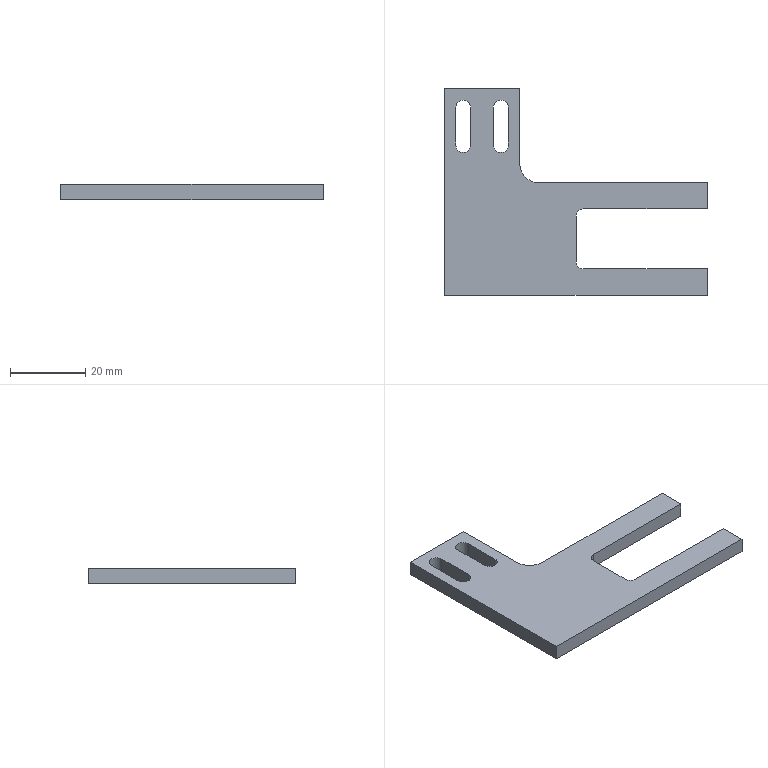Part | SolidWorks | features Fillet 2, ICE 2, Extrusion 1 | 1 solid | 23 faces | box 70 x 55 x 4 mm | volume 7768 mm3 | plane 16 | cylinder 7 | commonest cylinder face diameters 4 x6 10 x1
STEP:
#1=CARTESIAN_POINT('',(70.,-55.,0.));
#2=VERTEX_POINT('',#1);
#3=CARTESIAN_POINT('',(70.,-48.,0.));
#4=VERTEX_POINT('',#3);
#5=CARTESIAN_POINT('',(70.,-55.,0.));
#6=DIRECTION('',(0.,1.,0.));
#7=VECTOR('',#6,1000.);
#8=LINE('',#5,#7);
#9=EDGE_CURVE('',#2,#4,#8,.T.);
#10=ORIENTED_EDGE('',*,*,#9,.T.);
#11=CARTESIAN_POINT('',(70.,-48.,4.));
#12=VERTEX_POINT('',#11);
#13=CARTESIAN_POINT('',(70.,-48.,-0.001));
#14=DIRECTION('',(0.,0.,1.));
#15=VECTOR('',#14,1000.);
#16=LINE('',#13,#15);
#17=EDGE_CURVE('',#4,#12,#16,.T.);
#18=ORIENTED_EDGE('',*,*,#17,.T.);
#19=CARTESIAN_POINT('',(70.,-55.,4.));
#20=VERTEX_POINT('',#19);
#21=CARTESIAN_POINT('',(70.,-55.,4.));
#22=DIRECTION('',(0.,1.,0.));
#23=VECTOR('',#22,1000.);
#24=LINE('',#21,#23);
#25=EDGE_CURVE('',#20,#12,#24,.T.);
#26=ORIENTED_EDGE('',*,*,#25,.F.);
#27=CARTESIAN_POINT('',(70.,-55.,4.));
#28=DIRECTION('',(0.,0.,-1.));
#29=VECTOR('',#28,1000.);
#30=LINE('',#27,#29);
#31=EDGE_CURVE('',#20,#2,#30,.T.);
#32=ORIENTED_EDGE('',*,*,#31,.T.);
#33=EDGE_LOOP('',(#10,#18,#26,#32));
#34=FACE_OUTER_BOUND('',#33,.T.);
#35=CARTESIAN_POINT('',(70.,-55.,4.));
#36=DIRECTION('',(-1.,0.,0.));
#37=DIRECTION('',(0.,0.,1.));
#38=AXIS2_PLACEMENT_3D('',#35,#36,#37);
#39=PLANE('',#38);
#40=ADVANCED_FACE('',(#34),#39,.F.);
#41=CARTESIAN_POINT('',(20.,0.,0.));
#42=VERTEX_POINT('',#41);
#43=CARTESIAN_POINT('',(0.,0.,0.));
#44=VERTEX_POINT('',#43);
#45=CARTESIAN_POINT('',(20.,0.,0.));
#46=DIRECTION('',(-1.,0.,0.));
#47=VECTOR('',#46,1000.);
#48=LINE('',#45,#47);
#49=EDGE_CURVE('',#42,#44,#48,.T.);
#50=ORIENTED_EDGE('',*,*,#49,.T.);
#51=CARTESIAN_POINT('',(0.,0.,4.));
#52=VERTEX_POINT('',#51);
#53=CARTESIAN_POINT('',(0.,0.,4.));
#54=DIRECTION('',(0.,0.,-1.));
#55=VECTOR('',#54,1000.);
#56=LINE('',#53,#55);
#57=EDGE_CURVE('',#52,#44,#56,.T.);
#58=ORIENTED_EDGE('',*,*,#57,.F.);
#59=CARTESIAN_POINT('',(20.,0.,4.));
#60=VERTEX_POINT('',#59);
#61=CARTESIAN_POINT('',(20.,0.,4.));
#62=DIRECTION('',(-1.,0.,0.));
#63=VECTOR('',#62,1000.);
#64=LINE('',#61,#63);
#65=EDGE_CURVE('',#60,#52,#64,.T.);
#66=ORIENTED_EDGE('',*,*,#65,.F.);
#67=CARTESIAN_POINT('',(20.,0.,4.));
#68=DIRECTION('',(0.,0.,-1.));
#69=VECTOR('',#68,1000.);
#70=LINE('',#67,#69);
#71=EDGE_CURVE('',#60,#42,#70,.T.);
#72=ORIENTED_EDGE('',*,*,#71,.T.);
#73=EDGE_LOOP('',(#50,#58,#66,#72));
#74=FACE_OUTER_BOUND('',#73,.T.);
#75=CARTESIAN_POINT('',(20.,0.,4.));
#76=DIRECTION('',(0.,-1.,0.));
#77=DIRECTION('',(1.,0.,0.));
#78=AXIS2_PLACEMENT_3D('',#75,#76,#77);
#79=PLANE('',#78);
#80=ADVANCED_FACE('',(#74),#79,.F.);
#81=CARTESIAN_POINT('',(0.,-55.,0.));
#82=VERTEX_POINT('',#81);
#83=CARTESIAN_POINT('',(0.,0.,0.));
#84=DIRECTION('',(0.,-1.,0.));
#85=VECTOR('',#84,1000.);
#86=LINE('',#83,#85);
#87=EDGE_CURVE('',#44,#82,#86,.T.);
#88=ORIENTED_EDGE('',*,*,#87,.T.);
#89=CARTESIAN_POINT('',(0.,-55.,4.));
#90=VERTEX_POINT('',#89);
#91=CARTESIAN_POINT('',(0.,-55.,4.));
#92=DIRECTION('',(0.,0.,-1.));
#93=VECTOR('',#92,1000.);
#94=LINE('',#91,#93);
#95=EDGE_CURVE('',#90,#82,#94,.T.);
#96=ORIENTED_EDGE('',*,*,#95,.F.);
#97=CARTESIAN_POINT('',(0.,0.,4.));
#98=DIRECTION('',(0.,-1.,0.));
#99=VECTOR('',#98,1000.);
#100=LINE('',#97,#99);
#101=EDGE_CURVE('',#52,#90,#100,.T.);
#102=ORIENTED_EDGE('',*,*,#101,.F.);
#103=ORIENTED_EDGE('',*,*,#57,.T.);
#104=EDGE_LOOP('',(#88,#96,#102,#103));
#105=FACE_OUTER_BOUND('',#104,.T.);
#106=CARTESIAN_POINT('',(0.,0.,4.));
#107=DIRECTION('',(1.,0.,0.));
#108=DIRECTION('',(0.,1.,0.));
#109=AXIS2_PLACEMENT_3D('',#106,#107,#108);
#110=PLANE('',#109);
#111=ADVANCED_FACE('',(#105),#110,.F.);
#112=CARTESIAN_POINT('',(0.,-55.,0.));
#113=DIRECTION('',(1.,0.,0.));
#114=VECTOR('',#113,1000.);
#115=LINE('',#112,#114);
#116=EDGE_CURVE('',#82,#2,#115,.T.);
#117=ORIENTED_EDGE('',*,*,#116,.T.);
#118=ORIENTED_EDGE('',*,*,#31,.F.);
#119=CARTESIAN_POINT('',(0.,-55.,4.));
#120=DIRECTION('',(1.,0.,0.));
#121=VECTOR('',#120,1000.);
#122=LINE('',#119,#121);
#123=EDGE_CURVE('',#90,#20,#122,.T.);
#124=ORIENTED_EDGE('',*,*,#123,.F.);
#125=ORIENTED_EDGE('',*,*,#95,.T.);
#126=EDGE_LOOP('',(#117,#118,#124,#125));
#127=FACE_OUTER_BOUND('',#126,.T.);
#128=CARTESIAN_POINT('',(0.,-55.,4.));
#129=DIRECTION('',(0.,1.,0.));
#130=DIRECTION('',(0.,0.,1.));
#131=AXIS2_PLACEMENT_3D('',#128,#129,#130);
#132=PLANE('',#131);
#133=ADVANCED_FACE('',(#127),#132,.F.);
#134=CARTESIAN_POINT('',(70.,-32.,4.));
#135=VERTEX_POINT('',#134);
#136=CARTESIAN_POINT('',(70.,-25.,4.));
#137=VERTEX_POINT('',#136);
#138=CARTESIAN_POINT('',(70.,-55.,4.));
#139=DIRECTION('',(0.,1.,0.));
#140=VECTOR('',#139,1000.);
#141=LINE('',#138,#140);
#142=EDGE_CURVE('',#135,#137,#141,.T.);
#143=ORIENTED_EDGE('',*,*,#142,.F.);
#144=CARTESIAN_POINT('',(70.,-32.,0.));
#145=VERTEX_POINT('',#144);
#146=CARTESIAN_POINT('',(70.,-32.,-0.001));
#147=DIRECTION('',(0.,0.,1.));
#148=VECTOR('',#147,1000.);
#149=LINE('',#146,#148);
#150=EDGE_CURVE('',#145,#135,#149,.T.);
#151=ORIENTED_EDGE('',*,*,#150,.F.);
#152=CARTESIAN_POINT('',(70.,-25.,0.));
#153=VERTEX_POINT('',#152);
#154=CARTESIAN_POINT('',(70.,-55.,0.));
#155=DIRECTION('',(0.,1.,0.));
#156=VECTOR('',#155,1000.);
#157=LINE('',#154,#156);
#158=EDGE_CURVE('',#145,#153,#157,.T.);
#159=ORIENTED_EDGE('',*,*,#158,.T.);
#160=CARTESIAN_POINT('',(70.,-25.,4.));
#161=DIRECTION('',(0.,0.,-1.));
#162=VECTOR('',#161,1000.);
#163=LINE('',#160,#162);
#164=EDGE_CURVE('',#137,#153,#163,.T.);
#165=ORIENTED_EDGE('',*,*,#164,.F.);
#166=EDGE_LOOP('',(#143,#151,#159,#165));
#167=FACE_OUTER_BOUND('',#166,.T.);
#168=CARTESIAN_POINT('',(70.,-55.,4.));
#169=DIRECTION('',(-1.,0.,0.));
#170=DIRECTION('',(0.,0.,1.));
#171=AXIS2_PLACEMENT_3D('',#168,#169,#170);
#172=PLANE('',#171);
#173=ADVANCED_FACE('',(#167),#172,.F.);
#174=CARTESIAN_POINT('',(25.,-25.,0.));
#175=VERTEX_POINT('',#174);
#176=CARTESIAN_POINT('',(70.,-25.,0.));
#177=DIRECTION('',(-1.,0.,0.));
#178=VECTOR('',#177,1000.);
#179=LINE('',#176,#178);
#180=EDGE_CURVE('',#153,#175,#179,.T.);
#181=ORIENTED_EDGE('',*,*,#180,.T.);
#182=CARTESIAN_POINT('',(25.,-25.,4.));
#183=VERTEX_POINT('',#182);
#184=CARTESIAN_POINT('',(25.,-25.,4.));
#185=DIRECTION('',(0.,0.,1.));
#186=VECTOR('',#185,1000.);
#187=LINE('',#184,#186);
#188=EDGE_CURVE('',#175,#183,#187,.T.);
#189=ORIENTED_EDGE('',*,*,#188,.T.);
#190=CARTESIAN_POINT('',(70.,-25.,4.));
#191=DIRECTION('',(-1.,0.,0.));
#192=VECTOR('',#191,1000.);
#193=LINE('',#190,#192);
#194=EDGE_CURVE('',#137,#183,#193,.T.);
#195=ORIENTED_EDGE('',*,*,#194,.F.);
#196=ORIENTED_EDGE('',*,*,#164,.T.);
#197=EDGE_LOOP('',(#181,#189,#195,#196));
#198=FACE_OUTER_BOUND('',#197,.T.);
#199=CARTESIAN_POINT('',(70.,-25.,4.));
#200=DIRECTION('',(0.,-1.,0.));
#201=DIRECTION('',(1.,0.,0.));
#202=AXIS2_PLACEMENT_3D('',#199,#200,#201);
#203=PLANE('',#202);
#204=ADVANCED_FACE('',(#198),#203,.F.);
#205=CARTESIAN_POINT('',(20.,-20.,4.));
#206=VERTEX_POINT('',#205);
#207=CARTESIAN_POINT('',(20.,-25.,4.));
#208=DIRECTION('',(0.,1.,0.));
#209=VECTOR('',#208,1000.);
#210=LINE('',#207,#209);
#211=EDGE_CURVE('',#206,#60,#210,.T.);
#212=ORIENTED_EDGE('',*,*,#211,.F.);
#213=CARTESIAN_POINT('',(20.,-20.,0.));
#214=VERTEX_POINT('',#213);
#215=CARTESIAN_POINT('',(20.,-20.,0.));
#216=DIRECTION('',(0.,0.,-1.));
#217=VECTOR('',#216,1000.);
#218=LINE('',#215,#217);
#219=EDGE_CURVE('',#206,#214,#218,.T.);
#220=ORIENTED_EDGE('',*,*,#219,.T.);
#221=CARTESIAN_POINT('',(20.,-25.,0.));
#222=DIRECTION('',(0.,1.,0.));
#223=VECTOR('',#222,1000.);
#224=LINE('',#221,#223);
#225=EDGE_CURVE('',#214,#42,#224,.T.);
#226=ORIENTED_EDGE('',*,*,#225,.T.);
#227=ORIENTED_EDGE('',*,*,#71,.F.);
#228=EDGE_LOOP('',(#212,#220,#226,#227));
#229=FACE_OUTER_BOUND('',#228,.T.);
#230=CARTESIAN_POINT('',(20.,-25.,4.));
#231=DIRECTION('',(-1.,0.,0.));
#232=DIRECTION('',(0.,0.,1.));
#233=AXIS2_PLACEMENT_3D('',#230,#231,#232);
#234=PLANE('',#233);
#235=ADVANCED_FACE('',(#229),#234,.F.);
#236=CARTESIAN_POINT('',(37.,-48.,4.));
#237=VERTEX_POINT('',#236);
#238=CARTESIAN_POINT('',(70.,-48.,4.));
#239=DIRECTION('',(1.,0.,0.));
#240=VECTOR('',#239,1000.);
#241=LINE('',#238,#240);
#242=EDGE_CURVE('',#237,#12,#241,.T.);
#243=ORIENTED_EDGE('',*,*,#242,.F.);
#244=CARTESIAN_POINT('',(35.,-46.,4.));
#245=VERTEX_POINT('',#244);
#246=CARTESIAN_POINT('',(37.,-46.,4.));
#247=DIRECTION('',(0.,0.,-1.));
#248=DIRECTION('',(1.,0.,0.));
#249=AXIS2_PLACEMENT_3D('',#246,#247,#248);
#250=CIRCLE('',#249,2.);
#251=EDGE_CURVE('',#237,#245,#250,.T.);
#252=ORIENTED_EDGE('',*,*,#251,.T.);
#253=CARTESIAN_POINT('',(35.,-34.,4.));
#254=VERTEX_POINT('',#253);
#255=CARTESIAN_POINT('',(35.,-32.,4.));
#256=DIRECTION('',(0.,-1.,0.));
#257=VECTOR('',#256,1000.);
#258=LINE('',#255,#257);
#259=EDGE_CURVE('',#254,#245,#258,.T.);
#260=ORIENTED_EDGE('',*,*,#259,.F.);
#261=CARTESIAN_POINT('',(37.,-32.,4.));
#262=VERTEX_POINT('',#261);
#263=CARTESIAN_POINT('',(37.,-34.,4.));
#264=DIRECTION('',(0.,0.,-1.));
#265=DIRECTION('',(1.,0.,0.));
#266=AXIS2_PLACEMENT_3D('',#263,#264,#265);
#267=CIRCLE('',#266,2.);
#268=EDGE_CURVE('',#254,#262,#267,.T.);
#269=ORIENTED_EDGE('',*,*,#268,.T.);
#270=CARTESIAN_POINT('',(70.,-32.,4.));
#271=DIRECTION('',(-1.,0.,0.));
#272=VECTOR('',#271,1000.);
#273=LINE('',#270,#272);
#274=EDGE_CURVE('',#135,#262,#273,.T.);
#275=ORIENTED_EDGE('',*,*,#274,.F.);
#276=ORIENTED_EDGE('',*,*,#142,.T.);
#277=ORIENTED_EDGE('',*,*,#194,.T.);
#278=CARTESIAN_POINT('',(25.,-20.,4.));
#279=DIRECTION('',(0.,0.,-1.));
#280=DIRECTION('',(1.,0.,0.));
#281=AXIS2_PLACEMENT_3D('',#278,#279,#280);
#282=CIRCLE('',#281,5.);
#283=EDGE_CURVE('',#183,#206,#282,.T.);
#284=ORIENTED_EDGE('',*,*,#283,.T.);
#285=ORIENTED_EDGE('',*,*,#211,.T.);
#286=ORIENTED_EDGE('',*,*,#65,.T.);
#287=ORIENTED_EDGE('',*,*,#101,.T.);
#288=ORIENTED_EDGE('',*,*,#123,.T.);
#289=ORIENTED_EDGE('',*,*,#25,.T.);
#290=EDGE_LOOP('',(#243,#252,#260,#269,#275,#276,#277,#284,#285,#286,#287,#288,#289));
#291=FACE_OUTER_BOUND('',#290,.T.);
#292=CARTESIAN_POINT('',(3.,-15.,4.));
#293=VERTEX_POINT('',#292);
#294=CARTESIAN_POINT('',(7.,-15.,4.));
#295=VERTEX_POINT('',#294);
#296=CARTESIAN_POINT('',(5.,-15.,4.));
#297=DIRECTION('',(0.,0.,1.));
#298=DIRECTION('',(1.,0.,0.));
#299=AXIS2_PLACEMENT_3D('',#296,#297,#298);
#300=CIRCLE('',#299,2.);
#301=EDGE_CURVE('',#293,#295,#300,.T.);
#302=ORIENTED_EDGE('',*,*,#301,.F.);
#303=CARTESIAN_POINT('',(3.,-5.,4.));
#304=VERTEX_POINT('',#303);
#305=CARTESIAN_POINT('',(3.,-15.,4.));
#306=DIRECTION('',(0.,-1.,0.));
#307=VECTOR('',#306,1000.);
#308=LINE('',#305,#307);
#309=EDGE_CURVE('',#304,#293,#308,.T.);
#310=ORIENTED_EDGE('',*,*,#309,.F.);
#311=CARTESIAN_POINT('',(7.,-5.,4.));
#312=VERTEX_POINT('',#311);
#313=CARTESIAN_POINT('',(5.,-5.,4.));
#314=DIRECTION('',(0.,0.,1.));
#315=DIRECTION('',(1.,0.,0.));
#316=AXIS2_PLACEMENT_3D('',#313,#314,#315);
#317=CIRCLE('',#316,2.);
#318=EDGE_CURVE('',#312,#304,#317,.T.);
#319=ORIENTED_EDGE('',*,*,#318,.F.);
#320=CARTESIAN_POINT('',(7.,-15.,4.));
#321=DIRECTION('',(0.,1.,0.));
#322=VECTOR('',#321,1000.);
#323=LINE('',#320,#322);
#324=EDGE_CURVE('',#295,#312,#323,.T.);
#325=ORIENTED_EDGE('',*,*,#324,.F.);
#326=EDGE_LOOP('',(#302,#310,#319,#325));
#327=FACE_BOUND('',#326,.T.);
#328=CARTESIAN_POINT('',(13.,-15.,4.));
#329=VERTEX_POINT('',#328);
#330=CARTESIAN_POINT('',(17.,-15.,4.));
#331=VERTEX_POINT('',#330);
#332=CARTESIAN_POINT('',(15.,-15.,4.));
#333=DIRECTION('',(0.,0.,1.));
#334=DIRECTION('',(1.,0.,0.));
#335=AXIS2_PLACEMENT_3D('',#332,#333,#334);
#336=CIRCLE('',#335,2.);
#337=EDGE_CURVE('',#329,#331,#336,.T.);
#338=ORIENTED_EDGE('',*,*,#337,.F.);
#339=CARTESIAN_POINT('',(13.,-5.,4.));
#340=VERTEX_POINT('',#339);
#341=CARTESIAN_POINT('',(13.,-15.,4.));
#342=DIRECTION('',(0.,-1.,0.));
#343=VECTOR('',#342,1000.);
#344=LINE('',#341,#343);
#345=EDGE_CURVE('',#340,#329,#344,.T.);
#346=ORIENTED_EDGE('',*,*,#345,.F.);
#347=CARTESIAN_POINT('',(17.,-5.,4.));
#348=VERTEX_POINT('',#347);
#349=CARTESIAN_POINT('',(15.,-5.,4.));
#350=DIRECTION('',(0.,0.,1.));
#351=DIRECTION('',(1.,0.,0.));
#352=AXIS2_PLACEMENT_3D('',#349,#350,#351);
#353=CIRCLE('',#352,2.);
#354=EDGE_CURVE('',#348,#340,#353,.T.);
#355=ORIENTED_EDGE('',*,*,#354,.F.);
#356=CARTESIAN_POINT('',(17.,-15.,4.));
#357=DIRECTION('',(0.,1.,0.));
#358=VECTOR('',#357,1000.);
#359=LINE('',#356,#358);
#360=EDGE_CURVE('',#331,#348,#359,.T.);
#361=ORIENTED_EDGE('',*,*,#360,.F.);
#362=EDGE_LOOP('',(#338,#346,#355,#361));
#363=FACE_BOUND('',#362,.T.);
#364=CARTESIAN_POINT('',(0.,0.,4.));
#365=DIRECTION('',(0.,0.,1.));
#366=DIRECTION('',(1.,0.,0.));
#367=AXIS2_PLACEMENT_3D('',#364,#365,#366);
#368=PLANE('',#367);
#369=ADVANCED_FACE('',(#291,#327,#363),#368,.T.);
#370=CARTESIAN_POINT('',(3.,-15.,0.));
#371=VERTEX_POINT('',#370);
#372=CARTESIAN_POINT('',(3.,-5.,0.));
#373=VERTEX_POINT('',#372);
#374=CARTESIAN_POINT('',(3.,-15.,0.));
#375=DIRECTION('',(0.,1.,0.));
#376=VECTOR('',#375,1000.);
#377=LINE('',#374,#376);
#378=EDGE_CURVE('',#371,#373,#377,.T.);
#379=ORIENTED_EDGE('',*,*,#378,.F.);
#380=CARTESIAN_POINT('',(7.,-15.,0.));
#381=VERTEX_POINT('',#380);
#382=CARTESIAN_POINT('',(5.,-15.,0.));
#383=DIRECTION('',(0.,0.,-1.));
#384=DIRECTION('',(1.,0.,0.));
#385=AXIS2_PLACEMENT_3D('',#382,#383,#384);
#386=CIRCLE('',#385,2.);
#387=EDGE_CURVE('',#381,#371,#386,.T.);
#388=ORIENTED_EDGE('',*,*,#387,.F.);
#389=CARTESIAN_POINT('',(7.,-5.,0.));
#390=VERTEX_POINT('',#389);
#391=CARTESIAN_POINT('',(7.,-15.,0.));
#392=DIRECTION('',(0.,-1.,0.));
#393=VECTOR('',#392,1000.);
#394=LINE('',#391,#393);
#395=EDGE_CURVE('',#390,#381,#394,.T.);
#396=ORIENTED_EDGE('',*,*,#395,.F.);
#397=CARTESIAN_POINT('',(5.,-5.,0.));
#398=DIRECTION('',(0.,0.,-1.));
#399=DIRECTION('',(1.,0.,0.));
#400=AXIS2_PLACEMENT_3D('',#397,#398,#399);
#401=CIRCLE('',#400,2.);
#402=EDGE_CURVE('',#373,#390,#401,.T.);
#403=ORIENTED_EDGE('',*,*,#402,.F.);
#404=EDGE_LOOP('',(#379,#388,#396,#403));
#405=FACE_BOUND('',#404,.T.);
#406=CARTESIAN_POINT('',(13.,-15.,0.));
#407=VERTEX_POINT('',#406);
#408=CARTESIAN_POINT('',(13.,-5.,0.));
#409=VERTEX_POINT('',#408);
#410=CARTESIAN_POINT('',(13.,-15.,0.));
#411=DIRECTION('',(0.,1.,0.));
#412=VECTOR('',#411,1000.);
#413=LINE('',#410,#412);
#414=EDGE_CURVE('',#407,#409,#413,.T.);
#415=ORIENTED_EDGE('',*,*,#414,.F.);
#416=CARTESIAN_POINT('',(17.,-15.,0.));
#417=VERTEX_POINT('',#416);
#418=CARTESIAN_POINT('',(15.,-15.,0.));
#419=DIRECTION('',(0.,0.,-1.));
#420=DIRECTION('',(1.,0.,0.));
#421=AXIS2_PLACEMENT_3D('',#418,#419,#420);
#422=CIRCLE('',#421,2.);
#423=EDGE_CURVE('',#417,#407,#422,.T.);
#424=ORIENTED_EDGE('',*,*,#423,.F.);
#425=CARTESIAN_POINT('',(17.,-5.,0.));
#426=VERTEX_POINT('',#425);
#427=CARTESIAN_POINT('',(17.,-15.,0.));
#428=DIRECTION('',(0.,-1.,0.));
#429=VECTOR('',#428,1000.);
#430=LINE('',#427,#429);
#431=EDGE_CURVE('',#426,#417,#430,.T.);
#432=ORIENTED_EDGE('',*,*,#431,.F.);
#433=CARTESIAN_POINT('',(15.,-5.,0.));
#434=DIRECTION('',(0.,0.,-1.));
#435=DIRECTION('',(1.,0.,0.));
#436=AXIS2_PLACEMENT_3D('',#433,#434,#435);
#437=CIRCLE('',#436,2.);
#438=EDGE_CURVE('',#409,#426,#437,.T.);
#439=ORIENTED_EDGE('',*,*,#438,.F.);
#440=EDGE_LOOP('',(#415,#424,#432,#439));
#441=FACE_BOUND('',#440,.T.);
#442=CARTESIAN_POINT('',(35.,-46.,0.));
#443=VERTEX_POINT('',#442);
#444=CARTESIAN_POINT('',(35.,-34.,0.));
#445=VERTEX_POINT('',#444);
#446=CARTESIAN_POINT('',(35.,-32.,0.));
#447=DIRECTION('',(0.,1.,0.));
#448=VECTOR('',#447,1000.);
#449=LINE('',#446,#448);
#450=EDGE_CURVE('',#443,#445,#449,.T.);
#451=ORIENTED_EDGE('',*,*,#450,.F.);
#452=CARTESIAN_POINT('',(37.,-48.,0.));
#453=VERTEX_POINT('',#452);
#454=CARTESIAN_POINT('',(37.,-46.,0.));
#455=DIRECTION('',(0.,0.,1.));
#456=DIRECTION('',(1.,0.,0.));
#457=AXIS2_PLACEMENT_3D('',#454,#455,#456);
#458=CIRCLE('',#457,2.);
#459=EDGE_CURVE('',#443,#453,#458,.T.);
#460=ORIENTED_EDGE('',*,*,#459,.T.);
#461=CARTESIAN_POINT('',(70.,-48.,0.));
#462=DIRECTION('',(-1.,0.,0.));
#463=VECTOR('',#462,1000.);
#464=LINE('',#461,#463);
#465=EDGE_CURVE('',#4,#453,#464,.T.);
#466=ORIENTED_EDGE('',*,*,#465,.F.);
#467=ORIENTED_EDGE('',*,*,#9,.F.);
#468=ORIENTED_EDGE('',*,*,#116,.F.);
#469=ORIENTED_EDGE('',*,*,#87,.F.);
#470=ORIENTED_EDGE('',*,*,#49,.F.);
#471=ORIENTED_EDGE('',*,*,#225,.F.);
#472=CARTESIAN_POINT('',(25.,-20.,0.));
#473=DIRECTION('',(0.,0.,1.));
#474=DIRECTION('',(1.,0.,0.));
#475=AXIS2_PLACEMENT_3D('',#472,#473,#474);
#476=CIRCLE('',#475,5.);
#477=EDGE_CURVE('',#214,#175,#476,.T.);
#478=ORIENTED_EDGE('',*,*,#477,.T.);
#479=ORIENTED_EDGE('',*,*,#180,.F.);
#480=ORIENTED_EDGE('',*,*,#158,.F.);
#481=CARTESIAN_POINT('',(37.,-32.,0.));
#482=VERTEX_POINT('',#481);
#483=CARTESIAN_POINT('',(70.,-32.,0.));
#484=DIRECTION('',(1.,0.,0.));
#485=VECTOR('',#484,1000.);
#486=LINE('',#483,#485);
#487=EDGE_CURVE('',#482,#145,#486,.T.);
#488=ORIENTED_EDGE('',*,*,#487,.F.);
#489=CARTESIAN_POINT('',(37.,-34.,0.));
#490=DIRECTION('',(0.,0.,1.));
#491=DIRECTION('',(1.,0.,0.));
#492=AXIS2_PLACEMENT_3D('',#489,#490,#491);
#493=CIRCLE('',#492,2.);
#494=EDGE_CURVE('',#482,#445,#493,.T.);
#495=ORIENTED_EDGE('',*,*,#494,.T.);
#496=EDGE_LOOP('',(#451,#460,#466,#467,#468,#469,#470,#471,#478,#479,#480,#488,#495));
#497=FACE_OUTER_BOUND('',#496,.T.);
#498=CARTESIAN_POINT('',(0.,0.,0.));
#499=DIRECTION('',(0.,0.,1.));
#500=DIRECTION('',(1.,0.,0.));
#501=AXIS2_PLACEMENT_3D('',#498,#499,#500);
#502=PLANE('',#501);
#503=ADVANCED_FACE('',(#405,#441,#497),#502,.F.);
#504=ORIENTED_EDGE('',*,*,#423,.T.);
#505=CARTESIAN_POINT('',(13.,-15.,-0.001));
#506=DIRECTION('',(0.,0.,1.));
#507=VECTOR('',#506,1000.);
#508=LINE('',#505,#507);
#509=EDGE_CURVE('',#407,#329,#508,.T.);
#510=ORIENTED_EDGE('',*,*,#509,.T.);
#511=ORIENTED_EDGE('',*,*,#337,.T.);
#512=CARTESIAN_POINT('',(17.,-15.,-0.001));
#513=DIRECTION('',(0.,0.,1.));
#514=VECTOR('',#513,1000.);
#515=LINE('',#512,#514);
#516=EDGE_CURVE('',#417,#331,#515,.T.);
#517=ORIENTED_EDGE('',*,*,#516,.F.);
#518=EDGE_LOOP('',(#504,#510,#511,#517));
#519=FACE_OUTER_BOUND('',#518,.T.);
#520=CARTESIAN_POINT('',(15.,-15.,-0.001));
#521=DIRECTION('',(0.,0.,1.));
#522=DIRECTION('',(1.,0.,0.));
#523=AXIS2_PLACEMENT_3D('',#520,#521,#522);
#524=CYLINDRICAL_SURFACE('',#523,2.);
#525=ADVANCED_FACE('',(#519),#524,.F.);
#526=ORIENTED_EDGE('',*,*,#414,.T.);
#527=CARTESIAN_POINT('',(13.,-5.,-0.001));
#528=DIRECTION('',(0.,0.,1.));
#529=VECTOR('',#528,1000.);
#530=LINE('',#527,#529);
#531=EDGE_CURVE('',#409,#340,#530,.T.);
#532=ORIENTED_EDGE('',*,*,#531,.T.);
#533=ORIENTED_EDGE('',*,*,#345,.T.);
#534=ORIENTED_EDGE('',*,*,#509,.F.);
#535=EDGE_LOOP('',(#526,#532,#533,#534));
#536=FACE_OUTER_BOUND('',#535,.T.);
#537=CARTESIAN_POINT('',(13.,-15.,-0.001));
#538=DIRECTION('',(-1.,0.,0.));
#539=DIRECTION('',(0.,0.,1.));
#540=AXIS2_PLACEMENT_3D('',#537,#538,#539);
#541=PLANE('',#540);
#542=ADVANCED_FACE('',(#536),#541,.F.);
#543=ORIENTED_EDGE('',*,*,#438,.T.);
#544=CARTESIAN_POINT('',(17.,-5.,-0.001));
#545=DIRECTION('',(0.,0.,1.));
#546=VECTOR('',#545,1000.);
#547=LINE('',#544,#546);
#548=EDGE_CURVE('',#426,#348,#547,.T.);
#549=ORIENTED_EDGE('',*,*,#548,.T.);
#550=ORIENTED_EDGE('',*,*,#354,.T.);
#551=ORIENTED_EDGE('',*,*,#531,.F.);
#552=EDGE_LOOP('',(#543,#549,#550,#551));
#553=FACE_OUTER_BOUND('',#552,.T.);
#554=CARTESIAN_POINT('',(15.,-5.,-0.001));
#555=DIRECTION('',(0.,0.,1.));
#556=DIRECTION('',(1.,0.,0.));
#557=AXIS2_PLACEMENT_3D('',#554,#555,#556);
#558=CYLINDRICAL_SURFACE('',#557,2.);
#559=ADVANCED_FACE('',(#553),#558,.F.);
#560=ORIENTED_EDGE('',*,*,#431,.T.);
#561=ORIENTED_EDGE('',*,*,#516,.T.);
#562=ORIENTED_EDGE('',*,*,#360,.T.);
#563=ORIENTED_EDGE('',*,*,#548,.F.);
#564=EDGE_LOOP('',(#560,#561,#562,#563));
#565=FACE_OUTER_BOUND('',#564,.T.);
#566=CARTESIAN_POINT('',(17.,-15.,-0.001));
#567=DIRECTION('',(1.,0.,0.));
#568=DIRECTION('',(0.,0.,-1.));
#569=AXIS2_PLACEMENT_3D('',#566,#567,#568);
#570=PLANE('',#569);
#571=ADVANCED_FACE('',(#565),#570,.F.);
#572=ORIENTED_EDGE('',*,*,#387,.T.);
#573=CARTESIAN_POINT('',(3.,-15.,-0.001));
#574=DIRECTION('',(0.,0.,1.));
#575=VECTOR('',#574,1000.);
#576=LINE('',#573,#575);
#577=EDGE_CURVE('',#371,#293,#576,.T.);
#578=ORIENTED_EDGE('',*,*,#577,.T.);
#579=ORIENTED_EDGE('',*,*,#301,.T.);
#580=CARTESIAN_POINT('',(7.,-15.,-0.001));
#581=DIRECTION('',(0.,0.,1.));
#582=VECTOR('',#581,1000.);
#583=LINE('',#580,#582);
#584=EDGE_CURVE('',#381,#295,#583,.T.);
#585=ORIENTED_EDGE('',*,*,#584,.F.);
#586=EDGE_LOOP('',(#572,#578,#579,#585));
#587=FACE_OUTER_BOUND('',#586,.T.);
#588=CARTESIAN_POINT('',(5.,-15.,-0.001));
#589=DIRECTION('',(0.,0.,1.));
#590=DIRECTION('',(1.,0.,0.));
#591=AXIS2_PLACEMENT_3D('',#588,#589,#590);
#592=CYLINDRICAL_SURFACE('',#591,2.);
#593=ADVANCED_FACE('',(#587),#592,.F.);
#594=ORIENTED_EDGE('',*,*,#378,.T.);
#595=CARTESIAN_POINT('',(3.,-5.,-0.001));
#596=DIRECTION('',(0.,0.,1.));
#597=VECTOR('',#596,1000.);
#598=LINE('',#595,#597);
#599=EDGE_CURVE('',#373,#304,#598,.T.);
#600=ORIENTED_EDGE('',*,*,#599,.T.);
#601=ORIENTED_EDGE('',*,*,#309,.T.);
#602=ORIENTED_EDGE('',*,*,#577,.F.);
#603=EDGE_LOOP('',(#594,#600,#601,#602));
#604=FACE_OUTER_BOUND('',#603,.T.);
#605=CARTESIAN_POINT('',(3.,-15.,-0.001));
#606=DIRECTION('',(-1.,0.,0.));
#607=DIRECTION('',(0.,0.,1.));
#608=AXIS2_PLACEMENT_3D('',#605,#606,#607);
#609=PLANE('',#608);
#610=ADVANCED_FACE('',(#604),#609,.F.);
#611=ORIENTED_EDGE('',*,*,#402,.T.);
#612=CARTESIAN_POINT('',(7.,-5.,-0.001));
#613=DIRECTION('',(0.,0.,1.));
#614=VECTOR('',#613,1000.);
#615=LINE('',#612,#614);
#616=EDGE_CURVE('',#390,#312,#615,.T.);
#617=ORIENTED_EDGE('',*,*,#616,.T.);
#618=ORIENTED_EDGE('',*,*,#318,.T.);
#619=ORIENTED_EDGE('',*,*,#599,.F.);
#620=EDGE_LOOP('',(#611,#617,#618,#619));
#621=FACE_OUTER_BOUND('',#620,.T.);
#622=CARTESIAN_POINT('',(5.,-5.,-0.001));
#623=DIRECTION('',(0.,0.,1.));
#624=DIRECTION('',(1.,0.,0.));
#625=AXIS2_PLACEMENT_3D('',#622,#623,#624);
#626=CYLINDRICAL_SURFACE('',#625,2.);
#627=ADVANCED_FACE('',(#621),#626,.F.);
#628=ORIENTED_EDGE('',*,*,#395,.T.);
#629=ORIENTED_EDGE('',*,*,#584,.T.);
#630=ORIENTED_EDGE('',*,*,#324,.T.);
#631=ORIENTED_EDGE('',*,*,#616,.F.);
#632=EDGE_LOOP('',(#628,#629,#630,#631));
#633=FACE_OUTER_BOUND('',#632,.T.);
#634=CARTESIAN_POINT('',(7.,-15.,-0.001));
#635=DIRECTION('',(1.,0.,0.));
#636=DIRECTION('',(0.,1.,0.));
#637=AXIS2_PLACEMENT_3D('',#634,#635,#636);
#638=PLANE('',#637);
#639=ADVANCED_FACE('',(#633),#638,.F.);
#640=ORIENTED_EDGE('',*,*,#283,.F.);
#641=ORIENTED_EDGE('',*,*,#188,.F.);
#642=ORIENTED_EDGE('',*,*,#477,.F.);
#643=ORIENTED_EDGE('',*,*,#219,.F.);
#644=EDGE_LOOP('',(#640,#641,#642,#643));
#645=FACE_OUTER_BOUND('',#644,.T.);
#646=CARTESIAN_POINT('',(25.,-20.,4.));
#647=DIRECTION('',(0.,0.,1.));
#648=DIRECTION('',(1.,0.,0.));
#649=AXIS2_PLACEMENT_3D('',#646,#647,#648);
#650=CYLINDRICAL_SURFACE('',#649,5.);
#651=ADVANCED_FACE('',(#645),#650,.F.);
#652=ORIENTED_EDGE('',*,*,#465,.T.);
#653=CARTESIAN_POINT('',(37.,-48.,4.));
#654=DIRECTION('',(0.,0.,1.));
#655=VECTOR('',#654,1000.);
#656=LINE('',#653,#655);
#657=EDGE_CURVE('',#453,#237,#656,.T.);
#658=ORIENTED_EDGE('',*,*,#657,.T.);
#659=ORIENTED_EDGE('',*,*,#242,.T.);
#660=ORIENTED_EDGE('',*,*,#17,.F.);
#661=EDGE_LOOP('',(#652,#658,#659,#660));
#662=FACE_OUTER_BOUND('',#661,.T.);
#663=CARTESIAN_POINT('',(70.,-48.,-0.001));
#664=DIRECTION('',(0.,-1.,0.));
#665=DIRECTION('',(1.,0.,0.));
#666=AXIS2_PLACEMENT_3D('',#663,#664,#665);
#667=PLANE('',#666);
#668=ADVANCED_FACE('',(#662),#667,.F.);
#669=ORIENTED_EDGE('',*,*,#259,.T.);
#670=CARTESIAN_POINT('',(35.,-46.,0.));
#671=DIRECTION('',(0.,0.,-1.));
#672=VECTOR('',#671,1000.);
#673=LINE('',#670,#672);
#674=EDGE_CURVE('',#245,#443,#673,.T.);
#675=ORIENTED_EDGE('',*,*,#674,.T.);
#676=ORIENTED_EDGE('',*,*,#450,.T.);
#677=CARTESIAN_POINT('',(35.,-34.,4.));
#678=DIRECTION('',(0.,0.,1.));
#679=VECTOR('',#678,1000.);
#680=LINE('',#677,#679);
#681=EDGE_CURVE('',#445,#254,#680,.T.);
#682=ORIENTED_EDGE('',*,*,#681,.T.);
#683=EDGE_LOOP('',(#669,#675,#676,#682));
#684=FACE_OUTER_BOUND('',#683,.T.);
#685=CARTESIAN_POINT('',(35.,-32.,-0.001));
#686=DIRECTION('',(-1.,0.,0.));
#687=DIRECTION('',(0.,0.,1.));
#688=AXIS2_PLACEMENT_3D('',#685,#686,#687);
#689=PLANE('',#688);
#690=ADVANCED_FACE('',(#684),#689,.F.);
#691=ORIENTED_EDGE('',*,*,#274,.T.);
#692=CARTESIAN_POINT('',(37.,-32.,0.));
#693=DIRECTION('',(0.,0.,-1.));
#694=VECTOR('',#693,1000.);
#695=LINE('',#692,#694);
#696=EDGE_CURVE('',#262,#482,#695,.T.);
#697=ORIENTED_EDGE('',*,*,#696,.T.);
#698=ORIENTED_EDGE('',*,*,#487,.T.);
#699=ORIENTED_EDGE('',*,*,#150,.T.);
#700=EDGE_LOOP('',(#691,#697,#698,#699));
#701=FACE_OUTER_BOUND('',#700,.T.);
#702=CARTESIAN_POINT('',(70.,-32.,-0.001));
#703=DIRECTION('',(0.,1.,0.));
#704=DIRECTION('',(-1.,0.,0.));
#705=AXIS2_PLACEMENT_3D('',#702,#703,#704);
#706=PLANE('',#705);
#707=ADVANCED_FACE('',(#701),#706,.F.);
#708=ORIENTED_EDGE('',*,*,#459,.F.);
#709=ORIENTED_EDGE('',*,*,#674,.F.);
#710=ORIENTED_EDGE('',*,*,#251,.F.);
#711=ORIENTED_EDGE('',*,*,#657,.F.);
#712=EDGE_LOOP('',(#708,#709,#710,#711));
#713=FACE_OUTER_BOUND('',#712,.T.);
#714=CARTESIAN_POINT('',(37.,-46.,-0.001));
#715=DIRECTION('',(0.,0.,-1.));
#716=DIRECTION('',(-1.,0.,0.));
#717=AXIS2_PLACEMENT_3D('',#714,#715,#716);
#718=CYLINDRICAL_SURFACE('',#717,2.);
#719=ADVANCED_FACE('',(#713),#718,.F.);
#720=ORIENTED_EDGE('',*,*,#494,.F.);
#721=ORIENTED_EDGE('',*,*,#696,.F.);
#722=ORIENTED_EDGE('',*,*,#268,.F.);
#723=ORIENTED_EDGE('',*,*,#681,.F.);
#724=EDGE_LOOP('',(#720,#721,#722,#723));
#725=FACE_OUTER_BOUND('',#724,.T.);
#726=CARTESIAN_POINT('',(37.,-34.,-0.001));
#727=DIRECTION('',(0.,0.,-1.));
#728=DIRECTION('',(-1.,0.,0.));
#729=AXIS2_PLACEMENT_3D('',#726,#727,#728);
#730=CYLINDRICAL_SURFACE('',#729,2.);
#731=ADVANCED_FACE('',(#725),#730,.F.);
#732=CLOSED_SHELL('',(#40,#80,#111,#133,#173,#204,#235,#369,#503,#525,#542,#559,#571,#593,#610,#627,#639,#651,#668,#690,#707,#719,#731));
#733=MANIFOLD_SOLID_BREP('',#732);
#734=CARTESIAN_POINT('',(0.,0.,0.));
#735=DIRECTION('',(0.,0.,1.));
#736=DIRECTION('',(1.,0.,0.));
#737=AXIS2_PLACEMENT_3D('',#734,#735,#736);
#738=(LENGTH_UNIT()NAMED_UNIT(*)SI_UNIT(.MILLI.,.METRE.));
#739=UNCERTAINTY_MEASURE_WITH_UNIT(LENGTH_MEASURE(0.00001),#738,'','');
#740=(NAMED_UNIT(*)PLANE_ANGLE_UNIT()SI_UNIT($,.RADIAN.));
#741=(NAMED_UNIT(*)SI_UNIT($,.STERADIAN.)SOLID_ANGLE_UNIT());
#742=(GEOMETRIC_REPRESENTATION_CONTEXT(3)GLOBAL_UNCERTAINTY_ASSIGNED_CONTEXT((#739))GLOBAL_UNIT_ASSIGNED_CONTEXT((#738,#740,#741))REPRESENTATION_CONTEXT('',''));
#743=ADVANCED_BREP_SHAPE_REPRESENTATION('',(#733,#737),#742);